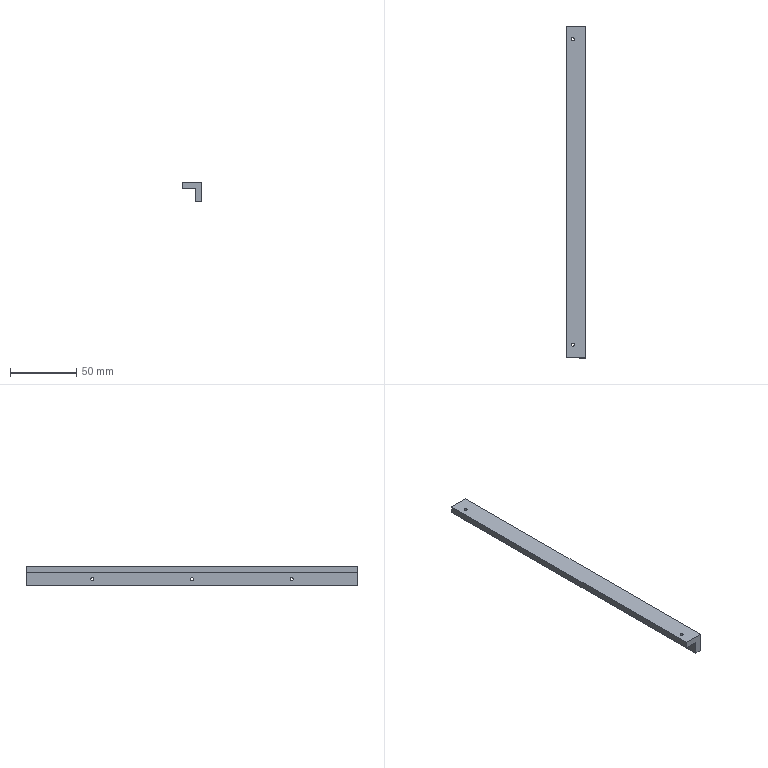Part | SolidWorks | features Cut 2, Extrusion 1 | 1 solid | 18 faces | box 15 x 250 x 15 mm | volume 31137 mm3 | cylinder 10 | plane 8 | commonest cylinder face diameters 2.4 x10
STEP:
#1=CARTESIAN_POINT('',(3.8,10.,-5.));
#2=VERTEX_POINT('',#1);
#3=CARTESIAN_POINT('',(6.2,10.,-5.));
#4=VERTEX_POINT('',#3);
#5=CARTESIAN_POINT('',(5.,10.,-5.));
#6=DIRECTION('',(0.,0.,1.));
#7=DIRECTION('',(1.,0.,0.));
#8=AXIS2_PLACEMENT_3D('',#5,#6,#7);
#9=CIRCLE('',#8,1.2);
#10=EDGE_CURVE('',#2,#4,#9,.T.);
#11=ORIENTED_EDGE('',*,*,#10,.F.);
#12=CARTESIAN_POINT('',(3.8,10.,0.));
#13=VERTEX_POINT('',#12);
#14=CARTESIAN_POINT('',(3.8,10.,-5.));
#15=DIRECTION('',(0.,0.,1.));
#16=VECTOR('',#15,1000.);
#17=LINE('',#14,#16);
#18=EDGE_CURVE('',#2,#13,#17,.T.);
#19=ORIENTED_EDGE('',*,*,#18,.T.);
#20=CARTESIAN_POINT('',(6.2,10.,0.));
#21=VERTEX_POINT('',#20);
#22=CARTESIAN_POINT('',(5.,10.,0.));
#23=DIRECTION('',(0.,0.,1.));
#24=DIRECTION('',(1.,0.,0.));
#25=AXIS2_PLACEMENT_3D('',#22,#23,#24);
#26=CIRCLE('',#25,1.2);
#27=EDGE_CURVE('',#13,#21,#26,.T.);
#28=ORIENTED_EDGE('',*,*,#27,.T.);
#29=CARTESIAN_POINT('',(6.2,10.,-5.));
#30=DIRECTION('',(0.,0.,1.));
#31=VECTOR('',#30,1000.);
#32=LINE('',#29,#31);
#33=EDGE_CURVE('',#4,#21,#32,.T.);
#34=ORIENTED_EDGE('',*,*,#33,.F.);
#35=EDGE_LOOP('',(#11,#19,#28,#34));
#36=FACE_OUTER_BOUND('',#35,.T.);
#37=CARTESIAN_POINT('',(5.,10.,-5.));
#38=DIRECTION('',(0.,0.,1.));
#39=DIRECTION('',(1.,0.,0.));
#40=AXIS2_PLACEMENT_3D('',#37,#38,#39);
#41=CYLINDRICAL_SURFACE('',#40,1.2);
#42=ADVANCED_FACE('',(#36),#41,.F.);
#43=CARTESIAN_POINT('',(3.8,240.,-5.));
#44=VERTEX_POINT('',#43);
#45=CARTESIAN_POINT('',(6.2,240.,-5.));
#46=VERTEX_POINT('',#45);
#47=CARTESIAN_POINT('',(5.,240.,-5.));
#48=DIRECTION('',(0.,0.,1.));
#49=DIRECTION('',(1.,0.,0.));
#50=AXIS2_PLACEMENT_3D('',#47,#48,#49);
#51=CIRCLE('',#50,1.2);
#52=EDGE_CURVE('',#44,#46,#51,.T.);
#53=ORIENTED_EDGE('',*,*,#52,.F.);
#54=CARTESIAN_POINT('',(3.8,240.,0.));
#55=VERTEX_POINT('',#54);
#56=CARTESIAN_POINT('',(3.8,240.,-5.));
#57=DIRECTION('',(0.,0.,1.));
#58=VECTOR('',#57,1000.);
#59=LINE('',#56,#58);
#60=EDGE_CURVE('',#44,#55,#59,.T.);
#61=ORIENTED_EDGE('',*,*,#60,.T.);
#62=CARTESIAN_POINT('',(6.2,240.,0.));
#63=VERTEX_POINT('',#62);
#64=CARTESIAN_POINT('',(5.,240.,0.));
#65=DIRECTION('',(0.,0.,1.));
#66=DIRECTION('',(1.,0.,0.));
#67=AXIS2_PLACEMENT_3D('',#64,#65,#66);
#68=CIRCLE('',#67,1.2);
#69=EDGE_CURVE('',#55,#63,#68,.T.);
#70=ORIENTED_EDGE('',*,*,#69,.T.);
#71=CARTESIAN_POINT('',(6.2,240.,-5.));
#72=DIRECTION('',(0.,0.,1.));
#73=VECTOR('',#72,1000.);
#74=LINE('',#71,#73);
#75=EDGE_CURVE('',#46,#63,#74,.T.);
#76=ORIENTED_EDGE('',*,*,#75,.F.);
#77=EDGE_LOOP('',(#53,#61,#70,#76));
#78=FACE_OUTER_BOUND('',#77,.T.);
#79=CARTESIAN_POINT('',(5.,240.,-5.));
#80=DIRECTION('',(0.,0.,1.));
#81=DIRECTION('',(1.,0.,0.));
#82=AXIS2_PLACEMENT_3D('',#79,#80,#81);
#83=CYLINDRICAL_SURFACE('',#82,1.2);
#84=ADVANCED_FACE('',(#78),#83,.F.);
#85=CARTESIAN_POINT('',(15.,50.,-11.2));
#86=VERTEX_POINT('',#85);
#87=CARTESIAN_POINT('',(15.,50.,-8.8));
#88=VERTEX_POINT('',#87);
#89=CARTESIAN_POINT('',(15.,50.,-10.));
#90=DIRECTION('',(-1.,0.,0.));
#91=DIRECTION('',(0.,0.,1.));
#92=AXIS2_PLACEMENT_3D('',#89,#90,#91);
#93=CIRCLE('',#92,1.2);
#94=EDGE_CURVE('',#86,#88,#93,.T.);
#95=ORIENTED_EDGE('',*,*,#94,.F.);
#96=CARTESIAN_POINT('',(10.,50.,-11.2));
#97=VERTEX_POINT('',#96);
#98=CARTESIAN_POINT('',(20.,50.,-11.2));
#99=DIRECTION('',(-1.,0.,0.));
#100=VECTOR('',#99,1000.);
#101=LINE('',#98,#100);
#102=EDGE_CURVE('',#86,#97,#101,.T.);
#103=ORIENTED_EDGE('',*,*,#102,.T.);
#104=CARTESIAN_POINT('',(10.,50.,-8.8));
#105=VERTEX_POINT('',#104);
#106=CARTESIAN_POINT('',(10.,50.,-10.));
#107=DIRECTION('',(-1.,0.,0.));
#108=DIRECTION('',(0.,0.,1.));
#109=AXIS2_PLACEMENT_3D('',#106,#107,#108);
#110=CIRCLE('',#109,1.2);
#111=EDGE_CURVE('',#97,#105,#110,.T.);
#112=ORIENTED_EDGE('',*,*,#111,.T.);
#113=CARTESIAN_POINT('',(20.,50.,-8.8));
#114=DIRECTION('',(-1.,0.,0.));
#115=VECTOR('',#114,1000.);
#116=LINE('',#113,#115);
#117=EDGE_CURVE('',#88,#105,#116,.T.);
#118=ORIENTED_EDGE('',*,*,#117,.F.);
#119=EDGE_LOOP('',(#95,#103,#112,#118));
#120=FACE_OUTER_BOUND('',#119,.T.);
#121=CARTESIAN_POINT('',(20.,50.,-10.));
#122=DIRECTION('',(-1.,0.,0.));
#123=DIRECTION('',(0.,0.,1.));
#124=AXIS2_PLACEMENT_3D('',#121,#122,#123);
#125=CYLINDRICAL_SURFACE('',#124,1.2);
#126=ADVANCED_FACE('',(#120),#125,.F.);
#127=CARTESIAN_POINT('',(15.,125.,-11.2));
#128=VERTEX_POINT('',#127);
#129=CARTESIAN_POINT('',(15.,125.,-8.8));
#130=VERTEX_POINT('',#129);
#131=CARTESIAN_POINT('',(15.,125.,-10.));
#132=DIRECTION('',(-1.,0.,0.));
#133=DIRECTION('',(0.,0.,1.));
#134=AXIS2_PLACEMENT_3D('',#131,#132,#133);
#135=CIRCLE('',#134,1.2);
#136=EDGE_CURVE('',#128,#130,#135,.T.);
#137=ORIENTED_EDGE('',*,*,#136,.F.);
#138=CARTESIAN_POINT('',(10.,125.,-11.2));
#139=VERTEX_POINT('',#138);
#140=CARTESIAN_POINT('',(20.,125.,-11.2));
#141=DIRECTION('',(-1.,0.,0.));
#142=VECTOR('',#141,1000.);
#143=LINE('',#140,#142);
#144=EDGE_CURVE('',#128,#139,#143,.T.);
#145=ORIENTED_EDGE('',*,*,#144,.T.);
#146=CARTESIAN_POINT('',(10.,125.,-8.8));
#147=VERTEX_POINT('',#146);
#148=CARTESIAN_POINT('',(10.,125.,-10.));
#149=DIRECTION('',(-1.,0.,0.));
#150=DIRECTION('',(0.,0.,1.));
#151=AXIS2_PLACEMENT_3D('',#148,#149,#150);
#152=CIRCLE('',#151,1.2);
#153=EDGE_CURVE('',#139,#147,#152,.T.);
#154=ORIENTED_EDGE('',*,*,#153,.T.);
#155=CARTESIAN_POINT('',(20.,125.,-8.8));
#156=DIRECTION('',(-1.,0.,0.));
#157=VECTOR('',#156,1000.);
#158=LINE('',#155,#157);
#159=EDGE_CURVE('',#130,#147,#158,.T.);
#160=ORIENTED_EDGE('',*,*,#159,.F.);
#161=EDGE_LOOP('',(#137,#145,#154,#160));
#162=FACE_OUTER_BOUND('',#161,.T.);
#163=CARTESIAN_POINT('',(20.,125.,-10.));
#164=DIRECTION('',(-1.,0.,0.));
#165=DIRECTION('',(0.,0.,1.));
#166=AXIS2_PLACEMENT_3D('',#163,#164,#165);
#167=CYLINDRICAL_SURFACE('',#166,1.2);
#168=ADVANCED_FACE('',(#162),#167,.F.);
#169=CARTESIAN_POINT('',(15.,200.,-11.2));
#170=VERTEX_POINT('',#169);
#171=CARTESIAN_POINT('',(15.,200.,-8.8));
#172=VERTEX_POINT('',#171);
#173=CARTESIAN_POINT('',(15.,200.,-10.));
#174=DIRECTION('',(-1.,0.,0.));
#175=DIRECTION('',(0.,0.,1.));
#176=AXIS2_PLACEMENT_3D('',#173,#174,#175);
#177=CIRCLE('',#176,1.2);
#178=EDGE_CURVE('',#170,#172,#177,.T.);
#179=ORIENTED_EDGE('',*,*,#178,.F.);
#180=CARTESIAN_POINT('',(10.,200.,-11.2));
#181=VERTEX_POINT('',#180);
#182=CARTESIAN_POINT('',(20.,200.,-11.2));
#183=DIRECTION('',(-1.,0.,0.));
#184=VECTOR('',#183,1000.);
#185=LINE('',#182,#184);
#186=EDGE_CURVE('',#170,#181,#185,.T.);
#187=ORIENTED_EDGE('',*,*,#186,.T.);
#188=CARTESIAN_POINT('',(10.,200.,-8.8));
#189=VERTEX_POINT('',#188);
#190=CARTESIAN_POINT('',(10.,200.,-10.));
#191=DIRECTION('',(-1.,0.,0.));
#192=DIRECTION('',(0.,0.,1.));
#193=AXIS2_PLACEMENT_3D('',#190,#191,#192);
#194=CIRCLE('',#193,1.2);
#195=EDGE_CURVE('',#181,#189,#194,.T.);
#196=ORIENTED_EDGE('',*,*,#195,.T.);
#197=CARTESIAN_POINT('',(20.,200.,-8.8));
#198=DIRECTION('',(-1.,0.,0.));
#199=VECTOR('',#198,1000.);
#200=LINE('',#197,#199);
#201=EDGE_CURVE('',#172,#189,#200,.T.);
#202=ORIENTED_EDGE('',*,*,#201,.F.);
#203=EDGE_LOOP('',(#179,#187,#196,#202));
#204=FACE_OUTER_BOUND('',#203,.T.);
#205=CARTESIAN_POINT('',(20.,200.,-10.));
#206=DIRECTION('',(-1.,0.,0.));
#207=DIRECTION('',(0.,0.,1.));
#208=AXIS2_PLACEMENT_3D('',#205,#206,#207);
#209=CYLINDRICAL_SURFACE('',#208,1.2);
#210=ADVANCED_FACE('',(#204),#209,.F.);
#211=CARTESIAN_POINT('',(0.,0.,-5.));
#212=VERTEX_POINT('',#211);
#213=CARTESIAN_POINT('',(0.,0.,0.));
#214=VERTEX_POINT('',#213);
#215=CARTESIAN_POINT('',(0.,0.,-5.));
#216=DIRECTION('',(0.,0.,1.));
#217=VECTOR('',#216,1000.);
#218=LINE('',#215,#217);
#219=EDGE_CURVE('',#212,#214,#218,.T.);
#220=ORIENTED_EDGE('',*,*,#219,.T.);
#221=CARTESIAN_POINT('',(0.,250.,0.));
#222=VERTEX_POINT('',#221);
#223=CARTESIAN_POINT('',(0.,250.,0.));
#224=DIRECTION('',(0.,-1.,0.));
#225=VECTOR('',#224,1000.);
#226=LINE('',#223,#225);
#227=EDGE_CURVE('',#222,#214,#226,.T.);
#228=ORIENTED_EDGE('',*,*,#227,.F.);
#229=CARTESIAN_POINT('',(0.,250.,-5.));
#230=VERTEX_POINT('',#229);
#231=CARTESIAN_POINT('',(0.,250.,-5.));
#232=DIRECTION('',(0.,0.,1.));
#233=VECTOR('',#232,1000.);
#234=LINE('',#231,#233);
#235=EDGE_CURVE('',#230,#222,#234,.T.);
#236=ORIENTED_EDGE('',*,*,#235,.F.);
#237=CARTESIAN_POINT('',(0.,250.,-5.));
#238=DIRECTION('',(0.,-1.,0.));
#239=VECTOR('',#238,1000.);
#240=LINE('',#237,#239);
#241=EDGE_CURVE('',#230,#212,#240,.T.);
#242=ORIENTED_EDGE('',*,*,#241,.T.);
#243=EDGE_LOOP('',(#220,#228,#236,#242));
#244=FACE_OUTER_BOUND('',#243,.T.);
#245=CARTESIAN_POINT('',(0.,250.,-5.));
#246=DIRECTION('',(1.,0.,0.));
#247=DIRECTION('',(0.,0.,-1.));
#248=AXIS2_PLACEMENT_3D('',#245,#246,#247);
#249=PLANE('',#248);
#250=ADVANCED_FACE('',(#244),#249,.F.);
#251=CARTESIAN_POINT('',(5.,10.,0.));
#252=DIRECTION('',(0.,0.,1.));
#253=DIRECTION('',(1.,0.,0.));
#254=AXIS2_PLACEMENT_3D('',#251,#252,#253);
#255=CIRCLE('',#254,1.2);
#256=EDGE_CURVE('',#21,#13,#255,.T.);
#257=ORIENTED_EDGE('',*,*,#256,.F.);
#258=ORIENTED_EDGE('',*,*,#27,.F.);
#259=EDGE_LOOP('',(#257,#258));
#260=FACE_BOUND('',#259,.T.);
#261=CARTESIAN_POINT('',(5.,240.,0.));
#262=DIRECTION('',(0.,0.,1.));
#263=DIRECTION('',(1.,0.,0.));
#264=AXIS2_PLACEMENT_3D('',#261,#262,#263);
#265=CIRCLE('',#264,1.2);
#266=EDGE_CURVE('',#63,#55,#265,.T.);
#267=ORIENTED_EDGE('',*,*,#266,.F.);
#268=ORIENTED_EDGE('',*,*,#69,.F.);
#269=EDGE_LOOP('',(#267,#268));
#270=FACE_BOUND('',#269,.T.);
#271=CARTESIAN_POINT('',(15.,0.,0.));
#272=VERTEX_POINT('',#271);
#273=CARTESIAN_POINT('',(0.,0.,0.));
#274=DIRECTION('',(1.,0.,0.));
#275=VECTOR('',#274,1000.);
#276=LINE('',#273,#275);
#277=EDGE_CURVE('',#214,#272,#276,.T.);
#278=ORIENTED_EDGE('',*,*,#277,.T.);
#279=CARTESIAN_POINT('',(15.,250.,0.));
#280=VERTEX_POINT('',#279);
#281=CARTESIAN_POINT('',(15.,250.,0.));
#282=DIRECTION('',(0.,-1.,0.));
#283=VECTOR('',#282,1000.);
#284=LINE('',#281,#283);
#285=EDGE_CURVE('',#280,#272,#284,.T.);
#286=ORIENTED_EDGE('',*,*,#285,.F.);
#287=CARTESIAN_POINT('',(0.,250.,0.));
#288=DIRECTION('',(1.,0.,0.));
#289=VECTOR('',#288,1000.);
#290=LINE('',#287,#289);
#291=EDGE_CURVE('',#222,#280,#290,.T.);
#292=ORIENTED_EDGE('',*,*,#291,.F.);
#293=ORIENTED_EDGE('',*,*,#227,.T.);
#294=EDGE_LOOP('',(#278,#286,#292,#293));
#295=FACE_OUTER_BOUND('',#294,.T.);
#296=CARTESIAN_POINT('',(0.,250.,0.));
#297=DIRECTION('',(0.,0.,-1.));
#298=DIRECTION('',(-1.,0.,0.));
#299=AXIS2_PLACEMENT_3D('',#296,#297,#298);
#300=PLANE('',#299);
#301=ADVANCED_FACE('',(#260,#270,#295),#300,.F.);
#302=CARTESIAN_POINT('',(15.,50.,-10.));
#303=DIRECTION('',(-1.,0.,0.));
#304=DIRECTION('',(0.,0.,1.));
#305=AXIS2_PLACEMENT_3D('',#302,#303,#304);
#306=CIRCLE('',#305,1.2);
#307=EDGE_CURVE('',#88,#86,#306,.T.);
#308=ORIENTED_EDGE('',*,*,#307,.T.);
#309=ORIENTED_EDGE('',*,*,#94,.T.);
#310=EDGE_LOOP('',(#308,#309));
#311=FACE_BOUND('',#310,.T.);
#312=CARTESIAN_POINT('',(15.,125.,-10.));
#313=DIRECTION('',(-1.,0.,0.));
#314=DIRECTION('',(0.,0.,1.));
#315=AXIS2_PLACEMENT_3D('',#312,#313,#314);
#316=CIRCLE('',#315,1.2);
#317=EDGE_CURVE('',#130,#128,#316,.T.);
#318=ORIENTED_EDGE('',*,*,#317,.T.);
#319=ORIENTED_EDGE('',*,*,#136,.T.);
#320=EDGE_LOOP('',(#318,#319));
#321=FACE_BOUND('',#320,.T.);
#322=CARTESIAN_POINT('',(15.,200.,-10.));
#323=DIRECTION('',(-1.,0.,0.));
#324=DIRECTION('',(0.,0.,1.));
#325=AXIS2_PLACEMENT_3D('',#322,#323,#324);
#326=CIRCLE('',#325,1.2);
#327=EDGE_CURVE('',#172,#170,#326,.T.);
#328=ORIENTED_EDGE('',*,*,#327,.T.);
#329=ORIENTED_EDGE('',*,*,#178,.T.);
#330=EDGE_LOOP('',(#328,#329));
#331=FACE_BOUND('',#330,.T.);
#332=CARTESIAN_POINT('',(15.,0.,-15.));
#333=VERTEX_POINT('',#332);
#334=CARTESIAN_POINT('',(15.,0.,0.));
#335=DIRECTION('',(0.,0.,-1.));
#336=VECTOR('',#335,1000.);
#337=LINE('',#334,#336);
#338=EDGE_CURVE('',#272,#333,#337,.T.);
#339=ORIENTED_EDGE('',*,*,#338,.T.);
#340=CARTESIAN_POINT('',(15.,250.,-15.));
#341=VERTEX_POINT('',#340);
#342=CARTESIAN_POINT('',(15.,250.,-15.));
#343=DIRECTION('',(0.,-1.,0.));
#344=VECTOR('',#343,1000.);
#345=LINE('',#342,#344);
#346=EDGE_CURVE('',#341,#333,#345,.T.);
#347=ORIENTED_EDGE('',*,*,#346,.F.);
#348=CARTESIAN_POINT('',(15.,250.,0.));
#349=DIRECTION('',(0.,0.,-1.));
#350=VECTOR('',#349,1000.);
#351=LINE('',#348,#350);
#352=EDGE_CURVE('',#280,#341,#351,.T.);
#353=ORIENTED_EDGE('',*,*,#352,.F.);
#354=ORIENTED_EDGE('',*,*,#285,.T.);
#355=EDGE_LOOP('',(#339,#347,#353,#354));
#356=FACE_OUTER_BOUND('',#355,.T.);
#357=CARTESIAN_POINT('',(15.,250.,0.));
#358=DIRECTION('',(-1.,0.,0.));
#359=DIRECTION('',(0.,0.,1.));
#360=AXIS2_PLACEMENT_3D('',#357,#358,#359);
#361=PLANE('',#360);
#362=ADVANCED_FACE('',(#311,#321,#331,#356),#361,.F.);
#363=CARTESIAN_POINT('',(10.,0.,-15.));
#364=VERTEX_POINT('',#363);
#365=CARTESIAN_POINT('',(15.,0.,-15.));
#366=DIRECTION('',(-1.,0.,0.));
#367=VECTOR('',#366,1000.);
#368=LINE('',#365,#367);
#369=EDGE_CURVE('',#333,#364,#368,.T.);
#370=ORIENTED_EDGE('',*,*,#369,.T.);
#371=CARTESIAN_POINT('',(10.,250.,-15.));
#372=VERTEX_POINT('',#371);
#373=CARTESIAN_POINT('',(10.,250.,-15.));
#374=DIRECTION('',(0.,-1.,0.));
#375=VECTOR('',#374,1000.);
#376=LINE('',#373,#375);
#377=EDGE_CURVE('',#372,#364,#376,.T.);
#378=ORIENTED_EDGE('',*,*,#377,.F.);
#379=CARTESIAN_POINT('',(15.,250.,-15.));
#380=DIRECTION('',(-1.,0.,0.));
#381=VECTOR('',#380,1000.);
#382=LINE('',#379,#381);
#383=EDGE_CURVE('',#341,#372,#382,.T.);
#384=ORIENTED_EDGE('',*,*,#383,.F.);
#385=ORIENTED_EDGE('',*,*,#346,.T.);
#386=EDGE_LOOP('',(#370,#378,#384,#385));
#387=FACE_OUTER_BOUND('',#386,.T.);
#388=CARTESIAN_POINT('',(15.,250.,-15.));
#389=DIRECTION('',(0.,0.,1.));
#390=DIRECTION('',(1.,0.,0.));
#391=AXIS2_PLACEMENT_3D('',#388,#389,#390);
#392=PLANE('',#391);
#393=ADVANCED_FACE('',(#387),#392,.F.);
#394=CARTESIAN_POINT('',(10.,50.,-10.));
#395=DIRECTION('',(-1.,0.,0.));
#396=DIRECTION('',(0.,0.,1.));
#397=AXIS2_PLACEMENT_3D('',#394,#395,#396);
#398=CIRCLE('',#397,1.2);
#399=EDGE_CURVE('',#105,#97,#398,.T.);
#400=ORIENTED_EDGE('',*,*,#399,.F.);
#401=ORIENTED_EDGE('',*,*,#111,.F.);
#402=EDGE_LOOP('',(#400,#401));
#403=FACE_BOUND('',#402,.T.);
#404=CARTESIAN_POINT('',(10.,125.,-10.));
#405=DIRECTION('',(-1.,0.,0.));
#406=DIRECTION('',(0.,0.,1.));
#407=AXIS2_PLACEMENT_3D('',#404,#405,#406);
#408=CIRCLE('',#407,1.2);
#409=EDGE_CURVE('',#147,#139,#408,.T.);
#410=ORIENTED_EDGE('',*,*,#409,.F.);
#411=ORIENTED_EDGE('',*,*,#153,.F.);
#412=EDGE_LOOP('',(#410,#411));
#413=FACE_BOUND('',#412,.T.);
#414=CARTESIAN_POINT('',(10.,200.,-10.));
#415=DIRECTION('',(-1.,0.,0.));
#416=DIRECTION('',(0.,0.,1.));
#417=AXIS2_PLACEMENT_3D('',#414,#415,#416);
#418=CIRCLE('',#417,1.2);
#419=EDGE_CURVE('',#189,#181,#418,.T.);
#420=ORIENTED_EDGE('',*,*,#419,.F.);
#421=ORIENTED_EDGE('',*,*,#195,.F.);
#422=EDGE_LOOP('',(#420,#421));
#423=FACE_BOUND('',#422,.T.);
#424=CARTESIAN_POINT('',(10.,0.,-5.));
#425=VERTEX_POINT('',#424);
#426=CARTESIAN_POINT('',(10.,0.,-15.));
#427=DIRECTION('',(0.,0.,1.));
#428=VECTOR('',#427,1000.);
#429=LINE('',#426,#428);
#430=EDGE_CURVE('',#364,#425,#429,.T.);
#431=ORIENTED_EDGE('',*,*,#430,.T.);
#432=CARTESIAN_POINT('',(10.,250.,-5.));
#433=VERTEX_POINT('',#432);
#434=CARTESIAN_POINT('',(10.,250.,-5.));
#435=DIRECTION('',(0.,-1.,0.));
#436=VECTOR('',#435,1000.);
#437=LINE('',#434,#436);
#438=EDGE_CURVE('',#433,#425,#437,.T.);
#439=ORIENTED_EDGE('',*,*,#438,.F.);
#440=CARTESIAN_POINT('',(10.,250.,-15.));
#441=DIRECTION('',(0.,0.,1.));
#442=VECTOR('',#441,1000.);
#443=LINE('',#440,#442);
#444=EDGE_CURVE('',#372,#433,#443,.T.);
#445=ORIENTED_EDGE('',*,*,#444,.F.);
#446=ORIENTED_EDGE('',*,*,#377,.T.);
#447=EDGE_LOOP('',(#431,#439,#445,#446));
#448=FACE_OUTER_BOUND('',#447,.T.);
#449=CARTESIAN_POINT('',(10.,250.,-15.));
#450=DIRECTION('',(1.,0.,0.));
#451=DIRECTION('',(0.,0.,-1.));
#452=AXIS2_PLACEMENT_3D('',#449,#450,#451);
#453=PLANE('',#452);
#454=ADVANCED_FACE('',(#403,#413,#423,#448),#453,.F.);
#455=CARTESIAN_POINT('',(5.,10.,-5.));
#456=DIRECTION('',(0.,0.,1.));
#457=DIRECTION('',(1.,0.,0.));
#458=AXIS2_PLACEMENT_3D('',#455,#456,#457);
#459=CIRCLE('',#458,1.2);
#460=EDGE_CURVE('',#4,#2,#459,.T.);
#461=ORIENTED_EDGE('',*,*,#460,.T.);
#462=ORIENTED_EDGE('',*,*,#10,.T.);
#463=EDGE_LOOP('',(#461,#462));
#464=FACE_BOUND('',#463,.T.);
#465=CARTESIAN_POINT('',(5.,240.,-5.));
#466=DIRECTION('',(0.,0.,1.));
#467=DIRECTION('',(1.,0.,0.));
#468=AXIS2_PLACEMENT_3D('',#465,#466,#467);
#469=CIRCLE('',#468,1.2);
#470=EDGE_CURVE('',#46,#44,#469,.T.);
#471=ORIENTED_EDGE('',*,*,#470,.T.);
#472=ORIENTED_EDGE('',*,*,#52,.T.);
#473=EDGE_LOOP('',(#471,#472));
#474=FACE_BOUND('',#473,.T.);
#475=CARTESIAN_POINT('',(10.,0.,-5.));
#476=DIRECTION('',(-1.,0.,0.));
#477=VECTOR('',#476,1000.);
#478=LINE('',#475,#477);
#479=EDGE_CURVE('',#425,#212,#478,.T.);
#480=ORIENTED_EDGE('',*,*,#479,.T.);
#481=ORIENTED_EDGE('',*,*,#241,.F.);
#482=CARTESIAN_POINT('',(10.,250.,-5.));
#483=DIRECTION('',(-1.,0.,0.));
#484=VECTOR('',#483,1000.);
#485=LINE('',#482,#484);
#486=EDGE_CURVE('',#433,#230,#485,.T.);
#487=ORIENTED_EDGE('',*,*,#486,.F.);
#488=ORIENTED_EDGE('',*,*,#438,.T.);
#489=EDGE_LOOP('',(#480,#481,#487,#488));
#490=FACE_OUTER_BOUND('',#489,.T.);
#491=CARTESIAN_POINT('',(10.,250.,-5.));
#492=DIRECTION('',(0.,0.,1.));
#493=DIRECTION('',(1.,0.,0.));
#494=AXIS2_PLACEMENT_3D('',#491,#492,#493);
#495=PLANE('',#494);
#496=ADVANCED_FACE('',(#464,#474,#490),#495,.F.);
#497=ORIENTED_EDGE('',*,*,#235,.T.);
#498=ORIENTED_EDGE('',*,*,#291,.T.);
#499=ORIENTED_EDGE('',*,*,#352,.T.);
#500=ORIENTED_EDGE('',*,*,#383,.T.);
#501=ORIENTED_EDGE('',*,*,#444,.T.);
#502=ORIENTED_EDGE('',*,*,#486,.T.);
#503=EDGE_LOOP('',(#497,#498,#499,#500,#501,#502));
#504=FACE_OUTER_BOUND('',#503,.T.);
#505=CARTESIAN_POINT('',(0.,250.,0.));
#506=DIRECTION('',(0.,1.,0.));
#507=DIRECTION('',(0.,0.,1.));
#508=AXIS2_PLACEMENT_3D('',#505,#506,#507);
#509=PLANE('',#508);
#510=ADVANCED_FACE('',(#504),#509,.T.);
#511=ORIENTED_EDGE('',*,*,#219,.F.);
#512=ORIENTED_EDGE('',*,*,#479,.F.);
#513=ORIENTED_EDGE('',*,*,#430,.F.);
#514=ORIENTED_EDGE('',*,*,#369,.F.);
#515=ORIENTED_EDGE('',*,*,#338,.F.);
#516=ORIENTED_EDGE('',*,*,#277,.F.);
#517=EDGE_LOOP('',(#511,#512,#513,#514,#515,#516));
#518=FACE_OUTER_BOUND('',#517,.T.);
#519=CARTESIAN_POINT('',(0.,0.,0.));
#520=DIRECTION('',(0.,1.,0.));
#521=DIRECTION('',(0.,0.,1.));
#522=AXIS2_PLACEMENT_3D('',#519,#520,#521);
#523=PLANE('',#522);
#524=ADVANCED_FACE('',(#518),#523,.F.);
#525=ORIENTED_EDGE('',*,*,#186,.F.);
#526=ORIENTED_EDGE('',*,*,#327,.F.);
#527=ORIENTED_EDGE('',*,*,#201,.T.);
#528=ORIENTED_EDGE('',*,*,#419,.T.);
#529=EDGE_LOOP('',(#525,#526,#527,#528));
#530=FACE_OUTER_BOUND('',#529,.T.);
#531=CARTESIAN_POINT('',(20.,200.,-10.));
#532=DIRECTION('',(-1.,0.,0.));
#533=DIRECTION('',(0.,0.,1.));
#534=AXIS2_PLACEMENT_3D('',#531,#532,#533);
#535=CYLINDRICAL_SURFACE('',#534,1.2);
#536=ADVANCED_FACE('',(#530),#535,.F.);
#537=ORIENTED_EDGE('',*,*,#144,.F.);
#538=ORIENTED_EDGE('',*,*,#317,.F.);
#539=ORIENTED_EDGE('',*,*,#159,.T.);
#540=ORIENTED_EDGE('',*,*,#409,.T.);
#541=EDGE_LOOP('',(#537,#538,#539,#540));
#542=FACE_OUTER_BOUND('',#541,.T.);
#543=CARTESIAN_POINT('',(20.,125.,-10.));
#544=DIRECTION('',(-1.,0.,0.));
#545=DIRECTION('',(0.,0.,1.));
#546=AXIS2_PLACEMENT_3D('',#543,#544,#545);
#547=CYLINDRICAL_SURFACE('',#546,1.2);
#548=ADVANCED_FACE('',(#542),#547,.F.);
#549=ORIENTED_EDGE('',*,*,#102,.F.);
#550=ORIENTED_EDGE('',*,*,#307,.F.);
#551=ORIENTED_EDGE('',*,*,#117,.T.);
#552=ORIENTED_EDGE('',*,*,#399,.T.);
#553=EDGE_LOOP('',(#549,#550,#551,#552));
#554=FACE_OUTER_BOUND('',#553,.T.);
#555=CARTESIAN_POINT('',(20.,50.,-10.));
#556=DIRECTION('',(-1.,0.,0.));
#557=DIRECTION('',(0.,0.,1.));
#558=AXIS2_PLACEMENT_3D('',#555,#556,#557);
#559=CYLINDRICAL_SURFACE('',#558,1.2);
#560=ADVANCED_FACE('',(#554),#559,.F.);
#561=ORIENTED_EDGE('',*,*,#60,.F.);
#562=ORIENTED_EDGE('',*,*,#470,.F.);
#563=ORIENTED_EDGE('',*,*,#75,.T.);
#564=ORIENTED_EDGE('',*,*,#266,.T.);
#565=EDGE_LOOP('',(#561,#562,#563,#564));
#566=FACE_OUTER_BOUND('',#565,.T.);
#567=CARTESIAN_POINT('',(5.,240.,-5.));
#568=DIRECTION('',(0.,0.,1.));
#569=DIRECTION('',(1.,0.,0.));
#570=AXIS2_PLACEMENT_3D('',#567,#568,#569);
#571=CYLINDRICAL_SURFACE('',#570,1.2);
#572=ADVANCED_FACE('',(#566),#571,.F.);
#573=ORIENTED_EDGE('',*,*,#18,.F.);
#574=ORIENTED_EDGE('',*,*,#460,.F.);
#575=ORIENTED_EDGE('',*,*,#33,.T.);
#576=ORIENTED_EDGE('',*,*,#256,.T.);
#577=EDGE_LOOP('',(#573,#574,#575,#576));
#578=FACE_OUTER_BOUND('',#577,.T.);
#579=CARTESIAN_POINT('',(5.,10.,-5.));
#580=DIRECTION('',(0.,0.,1.));
#581=DIRECTION('',(1.,0.,0.));
#582=AXIS2_PLACEMENT_3D('',#579,#580,#581);
#583=CYLINDRICAL_SURFACE('',#582,1.2);
#584=ADVANCED_FACE('',(#578),#583,.F.);
#585=CLOSED_SHELL('',(#42,#84,#126,#168,#210,#250,#301,#362,#393,#454,#496,#510,#524,#536,#548,#560,#572,#584));
#586=MANIFOLD_SOLID_BREP('',#585);
#587=CARTESIAN_POINT('',(0.,0.,0.));
#588=DIRECTION('',(0.,0.,1.));
#589=DIRECTION('',(1.,0.,0.));
#590=AXIS2_PLACEMENT_3D('',#587,#588,#589);
#591=(LENGTH_UNIT()NAMED_UNIT(*)SI_UNIT(.MILLI.,.METRE.));
#592=UNCERTAINTY_MEASURE_WITH_UNIT(LENGTH_MEASURE(0.00001),#591,'','');
#593=(NAMED_UNIT(*)PLANE_ANGLE_UNIT()SI_UNIT($,.RADIAN.));
#594=(NAMED_UNIT(*)SI_UNIT($,.STERADIAN.)SOLID_ANGLE_UNIT());
#595=(GEOMETRIC_REPRESENTATION_CONTEXT(3)GLOBAL_UNCERTAINTY_ASSIGNED_CONTEXT((#592))GLOBAL_UNIT_ASSIGNED_CONTEXT((#591,#593,#594))REPRESENTATION_CONTEXT('',''));
#596=ADVANCED_BREP_SHAPE_REPRESENTATION('',(#586,#590),#595);